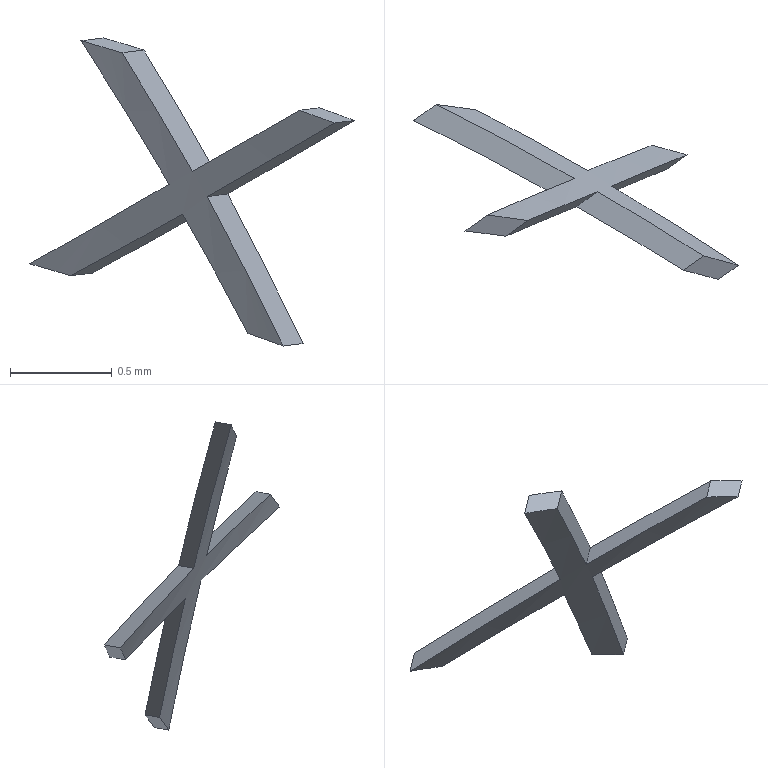Part | SolidWorks | features BaseBody 1 | 1 solid | 14 faces | box 1.595 x 0.8611 x 1.514 mm | volume 0.04844 mm3 | plane 12 | cylinder 2 | commonest cylinder face diameters 16.8 x1 17 x1
STEP:
#1=CARTESIAN_POINT('',(1968.242,-235.583,995.231));
#2=VERTEX_POINT('',#1);
#3=CARTESIAN_POINT('',(1968.793,-235.877,995.534));
#4=VERTEX_POINT('',#3);
#5=CARTESIAN_POINT('',(1968.242,-235.583,995.231));
#6=CARTESIAN_POINT('',(1968.429,-235.677,995.331));
#7=CARTESIAN_POINT('',(1968.612,-235.775,995.432));
#8=CARTESIAN_POINT('',(1968.793,-235.877,995.534));
#9=B_SPLINE_CURVE_WITH_KNOTS('',3,(#5,#6,#7,#8),.UNSPECIFIED.,.F.,.F.,(4,4),(0.,1.),.UNSPECIFIED.);
#10=EDGE_CURVE('',#2,#4,#9,.T.);
#11=ORIENTED_EDGE('',*,*,#10,.T.);
#12=CARTESIAN_POINT('',(1969.113,-235.75,994.948));
#13=VERTEX_POINT('',#12);
#14=CARTESIAN_POINT('',(1968.793,-235.877,995.534));
#15=CARTESIAN_POINT('',(1968.903,-235.832,995.341));
#16=CARTESIAN_POINT('',(1969.01,-235.79,995.145));
#17=CARTESIAN_POINT('',(1969.113,-235.75,994.948));
#18=B_SPLINE_CURVE_WITH_KNOTS('',3,(#14,#15,#16,#17),.UNSPECIFIED.,.F.,.F.,(4,4),(0.,1.),.UNSPECIFIED.);
#19=EDGE_CURVE('',#4,#13,#18,.T.);
#20=ORIENTED_EDGE('',*,*,#19,.T.);
#21=CARTESIAN_POINT('',(1969.287,-235.795,994.885));
#22=VERTEX_POINT('',#21);
#23=CARTESIAN_POINT('',(1966.247,-243.063,991.97));
#24=DIRECTION('',(-0.2015,0.436,-0.8771));
#25=DIRECTION('',(-0.7309,-0.6631,-0.1618));
#26=AXIS2_PLACEMENT_3D('',#23,#24,#25);
#27=CIRCLE('',#26,8.4);
#28=EDGE_CURVE('',#13,#22,#27,.T.);
#29=ORIENTED_EDGE('',*,*,#28,.T.);
#30=CARTESIAN_POINT('',(1968.912,-235.954,995.62));
#31=VERTEX_POINT('',#30);
#32=CARTESIAN_POINT('',(1968.912,-235.954,995.62));
#33=CARTESIAN_POINT('',(1969.042,-235.897,995.379));
#34=CARTESIAN_POINT('',(1969.167,-235.844,995.133));
#35=CARTESIAN_POINT('',(1969.287,-235.795,994.885));
#36=B_SPLINE_CURVE_WITH_KNOTS('',3,(#32,#33,#34,#35),.UNSPECIFIED.,.F.,.F.,(4,4),(0.,1.),.UNSPECIFIED.);
#37=EDGE_CURVE('',#31,#22,#36,.T.);
#38=ORIENTED_EDGE('',*,*,#37,.F.);
#39=CARTESIAN_POINT('',(1969.539,-236.34,995.982));
#40=VERTEX_POINT('',#39);
#41=CARTESIAN_POINT('',(1968.912,-235.954,995.62));
#42=CARTESIAN_POINT('',(1969.125,-236.077,995.74));
#43=CARTESIAN_POINT('',(1969.334,-236.206,995.861));
#44=CARTESIAN_POINT('',(1969.539,-236.34,995.982));
#45=B_SPLINE_CURVE_WITH_KNOTS('',3,(#41,#42,#43,#44),.UNSPECIFIED.,.F.,.F.,(4,4),(0.,1.),.UNSPECIFIED.);
#46=EDGE_CURVE('',#31,#40,#45,.T.);
#47=ORIENTED_EDGE('',*,*,#46,.T.);
#48=CARTESIAN_POINT('',(1969.365,-236.295,996.044));
#49=VERTEX_POINT('',#48);
#50=CARTESIAN_POINT('',(1966.499,-243.608,993.067));
#51=DIRECTION('',(0.2015,-0.436,0.8771));
#52=DIRECTION('',(-0.7309,-0.6631,-0.1618));
#53=AXIS2_PLACEMENT_3D('',#50,#51,#52);
#54=CIRCLE('',#53,8.4);
#55=EDGE_CURVE('',#40,#49,#54,.T.);
#56=ORIENTED_EDGE('',*,*,#55,.T.);
#57=CARTESIAN_POINT('',(1968.841,-235.982,995.744));
#58=VERTEX_POINT('',#57);
#59=CARTESIAN_POINT('',(1968.841,-235.982,995.744));
#60=CARTESIAN_POINT('',(1969.018,-236.082,995.844));
#61=CARTESIAN_POINT('',(1969.193,-236.187,995.944));
#62=CARTESIAN_POINT('',(1969.365,-236.295,996.044));
#63=B_SPLINE_CURVE_WITH_KNOTS('',3,(#59,#60,#61,#62),.UNSPECIFIED.,.F.,.F.,(4,4),(0.,1.),.UNSPECIFIED.);
#64=EDGE_CURVE('',#58,#49,#63,.T.);
#65=ORIENTED_EDGE('',*,*,#64,.F.);
#66=CARTESIAN_POINT('',(1968.494,-236.128,996.327));
#67=VERTEX_POINT('',#66);
#68=CARTESIAN_POINT('',(1968.494,-236.128,996.327));
#69=CARTESIAN_POINT('',(1968.613,-236.076,996.136));
#70=CARTESIAN_POINT('',(1968.729,-236.028,995.941));
#71=CARTESIAN_POINT('',(1968.841,-235.982,995.744));
#72=B_SPLINE_CURVE_WITH_KNOTS('',3,(#68,#69,#70,#71),.UNSPECIFIED.,.F.,.F.,(4,4),(0.,1.),.UNSPECIFIED.);
#73=EDGE_CURVE('',#67,#58,#72,.T.);
#74=ORIENTED_EDGE('',*,*,#73,.F.);
#75=CARTESIAN_POINT('',(1968.293,-236.103,996.386));
#76=VERTEX_POINT('',#75);
#77=CARTESIAN_POINT('',(1966.499,-243.608,993.067));
#78=DIRECTION('',(0.2015,-0.436,0.8771));
#79=DIRECTION('',(-0.7309,-0.6631,-0.1618));
#80=AXIS2_PLACEMENT_3D('',#77,#78,#79);
#81=CIRCLE('',#80,8.4);
#82=EDGE_CURVE('',#67,#76,#81,.T.);
#83=ORIENTED_EDGE('',*,*,#82,.T.);
#84=CARTESIAN_POINT('',(1968.726,-235.918,995.681));
#85=VERTEX_POINT('',#84);
#86=CARTESIAN_POINT('',(1968.293,-236.103,996.386));
#87=CARTESIAN_POINT('',(1968.442,-236.037,996.155));
#88=CARTESIAN_POINT('',(1968.587,-235.975,995.92));
#89=CARTESIAN_POINT('',(1968.726,-235.918,995.681));
#90=B_SPLINE_CURVE_WITH_KNOTS('',3,(#86,#87,#88,#89),.UNSPECIFIED.,.F.,.F.,(4,4),(0.,1.),.UNSPECIFIED.);
#91=EDGE_CURVE('',#76,#85,#90,.T.);
#92=ORIENTED_EDGE('',*,*,#91,.T.);
#93=CARTESIAN_POINT('',(1968.041,-235.558,995.289));
#94=VERTEX_POINT('',#93);
#95=CARTESIAN_POINT('',(1968.041,-235.558,995.289));
#96=CARTESIAN_POINT('',(1968.273,-235.671,995.419));
#97=CARTESIAN_POINT('',(1968.502,-235.791,995.55));
#98=CARTESIAN_POINT('',(1968.726,-235.918,995.681));
#99=B_SPLINE_CURVE_WITH_KNOTS('',3,(#95,#96,#97,#98),.UNSPECIFIED.,.F.,.F.,(4,4),(0.,1.),.UNSPECIFIED.);
#100=EDGE_CURVE('',#94,#85,#99,.T.);
#101=ORIENTED_EDGE('',*,*,#100,.F.);
#102=CARTESIAN_POINT('',(1966.247,-243.063,991.97));
#103=DIRECTION('',(-0.2015,0.436,-0.8771));
#104=DIRECTION('',(-0.7309,-0.6631,-0.1618));
#105=AXIS2_PLACEMENT_3D('',#102,#103,#104);
#106=CIRCLE('',#105,8.4);
#107=EDGE_CURVE('',#94,#2,#106,.T.);
#108=ORIENTED_EDGE('',*,*,#107,.T.);
#109=EDGE_LOOP('',(#11,#20,#29,#38,#47,#56,#65,#74,#83,#92,#101,#108));
#110=FACE_OUTER_BOUND('',#109,.T.);
#111=CARTESIAN_POINT('',(1967.45,-245.666,997.207));
#112=DIRECTION('',(0.2015,-0.436,0.8771));
#113=DIRECTION('',(-0.7309,-0.6631,-0.1618));
#114=AXIS2_PLACEMENT_3D('',#111,#112,#113);
#115=CYLINDRICAL_SURFACE('',#114,8.4);
#116=ADVANCED_FACE('',(#110),#115,.F.);
#117=CARTESIAN_POINT('',(1968.35,-235.506,995.244));
#118=VERTEX_POINT('',#117);
#119=CARTESIAN_POINT('',(1968.296,-235.544,995.237));
#120=DIRECTION('',(-0.8088,-0.5792,-0.1022));
#121=VECTOR('',#120,1000.);
#122=LINE('',#119,#121);
#123=EDGE_CURVE('',#118,#2,#122,.T.);
#124=ORIENTED_EDGE('',*,*,#123,.T.);
#125=ORIENTED_EDGE('',*,*,#107,.F.);
#126=CARTESIAN_POINT('',(1968.151,-235.479,995.303));
#127=VERTEX_POINT('',#126);
#128=CARTESIAN_POINT('',(1968.096,-235.518,995.296));
#129=DIRECTION('',(-0.8088,-0.5792,-0.1022));
#130=VECTOR('',#129,1000.);
#131=LINE('',#128,#130);
#132=EDGE_CURVE('',#127,#94,#131,.T.);
#133=ORIENTED_EDGE('',*,*,#132,.F.);
#134=CARTESIAN_POINT('',(1966.247,-243.063,991.97));
#135=DIRECTION('',(-0.2015,0.436,-0.8771));
#136=DIRECTION('',(-0.7309,-0.6631,-0.1618));
#137=AXIS2_PLACEMENT_3D('',#134,#135,#136);
#138=CIRCLE('',#137,8.5);
#139=EDGE_CURVE('',#127,#118,#138,.T.);
#140=ORIENTED_EDGE('',*,*,#139,.T.);
#141=EDGE_LOOP('',(#124,#125,#133,#140));
#142=FACE_OUTER_BOUND('',#141,.T.);
#143=CARTESIAN_POINT('',(1981.656,-238.46,990.719));
#144=DIRECTION('',(-0.2015,0.436,-0.8771));
#145=DIRECTION('',(-0.5526,0.6888,0.4693));
#146=AXIS2_PLACEMENT_3D('',#143,#144,#145);
#147=PLANE('',#146);
#148=ADVANCED_FACE('',(#142),#147,.T.);
#149=ORIENTED_EDGE('',*,*,#132,.T.);
#150=ORIENTED_EDGE('',*,*,#100,.T.);
#151=CARTESIAN_POINT('',(1968.83,-235.843,995.694));
#152=VERTEX_POINT('',#151);
#153=CARTESIAN_POINT('',(1968.778,-235.881,995.687));
#154=DIRECTION('',(-0.8088,-0.5792,-0.1022));
#155=VECTOR('',#154,1000.);
#156=LINE('',#153,#155);
#157=EDGE_CURVE('',#152,#85,#156,.T.);
#158=ORIENTED_EDGE('',*,*,#157,.F.);
#159=CARTESIAN_POINT('',(1968.151,-235.479,995.303));
#160=CARTESIAN_POINT('',(1968.289,-235.548,995.381));
#161=CARTESIAN_POINT('',(1968.426,-235.619,995.459));
#162=CARTESIAN_POINT('',(1968.562,-235.692,995.537));
#163=CARTESIAN_POINT('',(1968.696,-235.767,995.615));
#164=CARTESIAN_POINT('',(1968.83,-235.843,995.694));
#165=B_SPLINE_CURVE_WITH_KNOTS('',5,(#159,#160,#161,#162,#163,#164),.UNSPECIFIED.,.F.,.F.,(6,6),(0.,1.),.UNSPECIFIED.);
#166=EDGE_CURVE('',#127,#152,#165,.T.);
#167=ORIENTED_EDGE('',*,*,#166,.F.);
#168=EDGE_LOOP('',(#149,#150,#158,#167));
#169=FACE_OUTER_BOUND('',#168,.T.);
#170=CARTESIAN_POINT('',(1975.582,-231.008,996.547));
#171=DIRECTION('',(-0.3392,0.3175,0.8855));
#172=DIRECTION('',(0.4805,-0.7508,0.4532));
#173=AXIS2_PLACEMENT_3D('',#170,#171,#172);
#174=PLANE('',#173);
#175=ADVANCED_FACE('',(#169),#174,.T.);
#176=ORIENTED_EDGE('',*,*,#157,.T.);
#177=ORIENTED_EDGE('',*,*,#91,.F.);
#178=CARTESIAN_POINT('',(1968.403,-236.024,996.4));
#179=VERTEX_POINT('',#178);
#180=CARTESIAN_POINT('',(1968.348,-236.064,996.393));
#181=DIRECTION('',(-0.8088,-0.5792,-0.1022));
#182=VECTOR('',#181,1000.);
#183=LINE('',#180,#182);
#184=EDGE_CURVE('',#179,#76,#183,.T.);
#185=ORIENTED_EDGE('',*,*,#184,.F.);
#186=CARTESIAN_POINT('',(1968.403,-236.024,996.4));
#187=CARTESIAN_POINT('',(1968.491,-235.985,996.261));
#188=CARTESIAN_POINT('',(1968.578,-235.948,996.121));
#189=CARTESIAN_POINT('',(1968.664,-235.912,995.98));
#190=CARTESIAN_POINT('',(1968.747,-235.877,995.838));
#191=CARTESIAN_POINT('',(1968.83,-235.843,995.694));
#192=B_SPLINE_CURVE_WITH_KNOTS('',5,(#186,#187,#188,#189,#190,#191),.UNSPECIFIED.,.F.,.F.,(6,6),(0.,1.),.UNSPECIFIED.);
#193=EDGE_CURVE('',#179,#152,#192,.T.);
#194=ORIENTED_EDGE('',*,*,#193,.T.);
#195=EDGE_LOOP('',(#176,#177,#185,#194));
#196=FACE_OUTER_BOUND('',#195,.T.);
#197=CARTESIAN_POINT('',(1975.461,-230.969,997.291));
#198=DIRECTION('',(-0.5657,0.8136,-0.134));
#199=DIRECTION('',(-0.1608,0.05058,0.9857));
#200=AXIS2_PLACEMENT_3D('',#197,#198,#199);
#201=PLANE('',#200);
#202=ADVANCED_FACE('',(#196),#201,.T.);
#203=ORIENTED_EDGE('',*,*,#184,.T.);
#204=ORIENTED_EDGE('',*,*,#82,.F.);
#205=CARTESIAN_POINT('',(1968.602,-236.051,996.341));
#206=VERTEX_POINT('',#205);
#207=CARTESIAN_POINT('',(1968.548,-236.09,996.334));
#208=DIRECTION('',(-0.8088,-0.5792,-0.1022));
#209=VECTOR('',#208,1000.);
#210=LINE('',#207,#209);
#211=EDGE_CURVE('',#206,#67,#210,.T.);
#212=ORIENTED_EDGE('',*,*,#211,.F.);
#213=CARTESIAN_POINT('',(1966.499,-243.608,993.067));
#214=DIRECTION('',(0.2015,-0.436,0.8771));
#215=DIRECTION('',(-0.7309,-0.6631,-0.1618));
#216=AXIS2_PLACEMENT_3D('',#213,#214,#215);
#217=CIRCLE('',#216,8.5);
#218=EDGE_CURVE('',#206,#179,#217,.T.);
#219=ORIENTED_EDGE('',*,*,#218,.T.);
#220=EDGE_LOOP('',(#203,#204,#212,#219));
#221=FACE_OUTER_BOUND('',#220,.T.);
#222=CARTESIAN_POINT('',(1982.253,-239.435,991.522));
#223=DIRECTION('',(0.2015,-0.436,0.8771));
#224=DIRECTION('',(0.5526,-0.6888,-0.4693));
#225=AXIS2_PLACEMENT_3D('',#222,#223,#224);
#226=PLANE('',#225);
#227=ADVANCED_FACE('',(#221),#226,.T.);
#228=ORIENTED_EDGE('',*,*,#211,.T.);
#229=ORIENTED_EDGE('',*,*,#73,.T.);
#230=CARTESIAN_POINT('',(1968.944,-235.908,995.757));
#231=VERTEX_POINT('',#230);
#232=CARTESIAN_POINT('',(1968.893,-235.945,995.75));
#233=DIRECTION('',(-0.8088,-0.5792,-0.1022));
#234=VECTOR('',#233,1000.);
#235=LINE('',#232,#234);
#236=EDGE_CURVE('',#231,#58,#235,.T.);
#237=ORIENTED_EDGE('',*,*,#236,.F.);
#238=CARTESIAN_POINT('',(1968.602,-236.051,996.341));
#239=CARTESIAN_POINT('',(1968.672,-236.021,996.226));
#240=CARTESIAN_POINT('',(1968.742,-235.991,996.11));
#241=CARTESIAN_POINT('',(1968.81,-235.963,995.993));
#242=CARTESIAN_POINT('',(1968.878,-235.935,995.875));
#243=CARTESIAN_POINT('',(1968.944,-235.908,995.757));
#244=B_SPLINE_CURVE_WITH_KNOTS('',5,(#238,#239,#240,#241,#242,#243),.UNSPECIFIED.,.F.,.F.,(6,6),(0.,1.),.UNSPECIFIED.);
#245=EDGE_CURVE('',#206,#231,#244,.T.);
#246=ORIENTED_EDGE('',*,*,#245,.F.);
#247=EDGE_LOOP('',(#228,#229,#237,#246));
#248=FACE_OUTER_BOUND('',#247,.T.);
#249=CARTESIAN_POINT('',(1975.647,-231.108,996.604));
#250=DIRECTION('',(0.566,-0.8137,0.1326));
#251=DIRECTION('',(0.1599,-0.04938,-0.9859));
#252=AXIS2_PLACEMENT_3D('',#249,#250,#251);
#253=PLANE('',#252);
#254=ADVANCED_FACE('',(#248),#253,.T.);
#255=ORIENTED_EDGE('',*,*,#236,.T.);
#256=ORIENTED_EDGE('',*,*,#64,.T.);
#257=CARTESIAN_POINT('',(1969.464,-236.224,996.056));
#258=VERTEX_POINT('',#257);
#259=CARTESIAN_POINT('',(1969.415,-236.26,996.05));
#260=DIRECTION('',(-0.8088,-0.5792,-0.1022));
#261=VECTOR('',#260,1000.);
#262=LINE('',#259,#261);
#263=EDGE_CURVE('',#258,#49,#262,.T.);
#264=ORIENTED_EDGE('',*,*,#263,.F.);
#265=CARTESIAN_POINT('',(1968.944,-235.908,995.757));
#266=CARTESIAN_POINT('',(1969.05,-235.969,995.817));
#267=CARTESIAN_POINT('',(1969.154,-236.031,995.876));
#268=CARTESIAN_POINT('',(1969.258,-236.094,995.936));
#269=CARTESIAN_POINT('',(1969.362,-236.159,995.996));
#270=CARTESIAN_POINT('',(1969.464,-236.224,996.056));
#271=B_SPLINE_CURVE_WITH_KNOTS('',5,(#265,#266,#267,#268,#269,#270),.UNSPECIFIED.,.F.,.F.,(6,6),(0.,1.),.UNSPECIFIED.);
#272=EDGE_CURVE('',#231,#258,#271,.T.);
#273=ORIENTED_EDGE('',*,*,#272,.F.);
#274=EDGE_LOOP('',(#255,#256,#264,#273));
#275=FACE_OUTER_BOUND('',#274,.T.);
#276=CARTESIAN_POINT('',(1975.95,-231.579,996.876));
#277=DIRECTION('',(-0.3302,0.3034,0.8938));
#278=DIRECTION('',(0.4867,-0.7566,0.4367));
#279=AXIS2_PLACEMENT_3D('',#276,#277,#278);
#280=PLANE('',#279);
#281=ADVANCED_FACE('',(#275),#280,.T.);
#282=ORIENTED_EDGE('',*,*,#263,.T.);
#283=ORIENTED_EDGE('',*,*,#55,.F.);
#284=CARTESIAN_POINT('',(1969.636,-236.27,995.994));
#285=VERTEX_POINT('',#284);
#286=CARTESIAN_POINT('',(1969.587,-236.305,995.988));
#287=DIRECTION('',(-0.8088,-0.5792,-0.1022));
#288=VECTOR('',#287,1000.);
#289=LINE('',#286,#288);
#290=EDGE_CURVE('',#285,#40,#289,.T.);
#291=ORIENTED_EDGE('',*,*,#290,.F.);
#292=CARTESIAN_POINT('',(1966.499,-243.608,993.067));
#293=DIRECTION('',(0.2015,-0.436,0.8771));
#294=DIRECTION('',(-0.7309,-0.6631,-0.1618));
#295=AXIS2_PLACEMENT_3D('',#292,#293,#294);
#296=CIRCLE('',#295,8.5);
#297=EDGE_CURVE('',#285,#258,#296,.T.);
#298=ORIENTED_EDGE('',*,*,#297,.T.);
#299=EDGE_LOOP('',(#282,#283,#291,#298));
#300=FACE_OUTER_BOUND('',#299,.T.);
#301=CARTESIAN_POINT('',(1982.253,-239.435,991.522));
#302=DIRECTION('',(0.2015,-0.436,0.8771));
#303=DIRECTION('',(0.5526,-0.6888,-0.4693));
#304=AXIS2_PLACEMENT_3D('',#301,#302,#303);
#305=PLANE('',#304);
#306=ADVANCED_FACE('',(#300),#305,.T.);
#307=ORIENTED_EDGE('',*,*,#290,.T.);
#308=ORIENTED_EDGE('',*,*,#46,.F.);
#309=CARTESIAN_POINT('',(1969.014,-235.881,995.633));
#310=VERTEX_POINT('',#309);
#311=CARTESIAN_POINT('',(1968.963,-235.917,995.627));
#312=DIRECTION('',(-0.8088,-0.5792,-0.1022));
#313=VECTOR('',#312,1000.);
#314=LINE('',#311,#313);
#315=EDGE_CURVE('',#310,#31,#314,.T.);
#316=ORIENTED_EDGE('',*,*,#315,.F.);
#317=CARTESIAN_POINT('',(1969.014,-235.881,995.633));
#318=CARTESIAN_POINT('',(1969.141,-235.955,995.705));
#319=CARTESIAN_POINT('',(1969.266,-236.032,995.777));
#320=CARTESIAN_POINT('',(1969.391,-236.11,995.849));
#321=CARTESIAN_POINT('',(1969.514,-236.189,995.922));
#322=CARTESIAN_POINT('',(1969.636,-236.27,995.994));
#323=B_SPLINE_CURVE_WITH_KNOTS('',5,(#317,#318,#319,#320,#321,#322),.UNSPECIFIED.,.F.,.F.,(6,6),(0.,1.),.UNSPECIFIED.);
#324=EDGE_CURVE('',#310,#285,#323,.T.);
#325=ORIENTED_EDGE('',*,*,#324,.T.);
#326=EDGE_LOOP('',(#307,#308,#316,#325));
#327=FACE_OUTER_BOUND('',#326,.T.);
#328=CARTESIAN_POINT('',(1975.669,-231.115,996.474));
#329=DIRECTION('',(0.3295,-0.3023,-0.8944));
#330=DIRECTION('',(-0.4872,0.7571,-0.4354));
#331=AXIS2_PLACEMENT_3D('',#328,#329,#330);
#332=PLANE('',#331);
#333=ADVANCED_FACE('',(#327),#332,.T.);
#334=ORIENTED_EDGE('',*,*,#315,.T.);
#335=ORIENTED_EDGE('',*,*,#37,.T.);
#336=CARTESIAN_POINT('',(1969.384,-235.725,994.898));
#337=VERTEX_POINT('',#336);
#338=CARTESIAN_POINT('',(1969.336,-235.76,994.891));
#339=DIRECTION('',(-0.8088,-0.5792,-0.1022));
#340=VECTOR('',#339,1000.);
#341=LINE('',#338,#340);
#342=EDGE_CURVE('',#337,#22,#341,.T.);
#343=ORIENTED_EDGE('',*,*,#342,.F.);
#344=CARTESIAN_POINT('',(1969.014,-235.881,995.633));
#345=CARTESIAN_POINT('',(1969.091,-235.848,995.488));
#346=CARTESIAN_POINT('',(1969.166,-235.815,995.342));
#347=CARTESIAN_POINT('',(1969.24,-235.784,995.194));
#348=CARTESIAN_POINT('',(1969.313,-235.754,995.046));
#349=CARTESIAN_POINT('',(1969.384,-235.725,994.898));
#350=B_SPLINE_CURVE_WITH_KNOTS('',5,(#344,#345,#346,#347,#348,#349),.UNSPECIFIED.,.F.,.F.,(6,6),(0.,1.),.UNSPECIFIED.);
#351=EDGE_CURVE('',#310,#337,#350,.T.);
#352=ORIENTED_EDGE('',*,*,#351,.F.);
#353=EDGE_LOOP('',(#334,#335,#343,#352));
#354=FACE_OUTER_BOUND('',#353,.T.);
#355=CARTESIAN_POINT('',(1975.785,-231.142,995.706));
#356=DIRECTION('',(0.5689,-0.8145,0.1142));
#357=DIRECTION('',(0.1494,-0.03424,-0.9882));
#358=AXIS2_PLACEMENT_3D('',#355,#356,#357);
#359=PLANE('',#358);
#360=ADVANCED_FACE('',(#354),#359,.T.);
#361=ORIENTED_EDGE('',*,*,#342,.T.);
#362=ORIENTED_EDGE('',*,*,#28,.F.);
#363=CARTESIAN_POINT('',(1969.212,-235.679,994.96));
#364=VERTEX_POINT('',#363);
#365=CARTESIAN_POINT('',(1969.163,-235.715,994.954));
#366=DIRECTION('',(-0.8088,-0.5792,-0.1022));
#367=VECTOR('',#366,1000.);
#368=LINE('',#365,#367);
#369=EDGE_CURVE('',#364,#13,#368,.T.);
#370=ORIENTED_EDGE('',*,*,#369,.F.);
#371=CARTESIAN_POINT('',(1966.247,-243.063,991.97));
#372=DIRECTION('',(-0.2015,0.436,-0.8771));
#373=DIRECTION('',(-0.7309,-0.6631,-0.1618));
#374=AXIS2_PLACEMENT_3D('',#371,#372,#373);
#375=CIRCLE('',#374,8.5);
#376=EDGE_CURVE('',#364,#337,#375,.T.);
#377=ORIENTED_EDGE('',*,*,#376,.T.);
#378=EDGE_LOOP('',(#361,#362,#370,#377));
#379=FACE_OUTER_BOUND('',#378,.T.);
#380=CARTESIAN_POINT('',(1981.656,-238.46,990.719));
#381=DIRECTION('',(-0.2015,0.436,-0.8771));
#382=DIRECTION('',(-0.5526,0.6888,0.4693));
#383=AXIS2_PLACEMENT_3D('',#380,#381,#382);
#384=PLANE('',#383);
#385=ADVANCED_FACE('',(#379),#384,.T.);
#386=ORIENTED_EDGE('',*,*,#369,.T.);
#387=ORIENTED_EDGE('',*,*,#19,.F.);
#388=CARTESIAN_POINT('',(1968.896,-235.804,995.547));
#389=VERTEX_POINT('',#388);
#390=CARTESIAN_POINT('',(1968.844,-235.841,995.541));
#391=DIRECTION('',(-0.8088,-0.5792,-0.1022));
#392=VECTOR('',#391,1000.);
#393=LINE('',#390,#392);
#394=EDGE_CURVE('',#389,#4,#393,.T.);
#395=ORIENTED_EDGE('',*,*,#394,.F.);
#396=CARTESIAN_POINT('',(1968.896,-235.804,995.547));
#397=CARTESIAN_POINT('',(1968.961,-235.777,995.431));
#398=CARTESIAN_POINT('',(1969.025,-235.752,995.314));
#399=CARTESIAN_POINT('',(1969.088,-235.727,995.197));
#400=CARTESIAN_POINT('',(1969.151,-235.703,995.079));
#401=CARTESIAN_POINT('',(1969.212,-235.679,994.96));
#402=B_SPLINE_CURVE_WITH_KNOTS('',5,(#396,#397,#398,#399,#400,#401),.UNSPECIFIED.,.F.,.F.,(6,6),(0.,1.),.UNSPECIFIED.);
#403=EDGE_CURVE('',#389,#364,#402,.T.);
#404=ORIENTED_EDGE('',*,*,#403,.T.);
#405=EDGE_LOOP('',(#386,#387,#395,#404));
#406=FACE_OUTER_BOUND('',#405,.T.);
#407=CARTESIAN_POINT('',(1975.599,-231.003,996.394));
#408=DIRECTION('',(-0.566,0.8137,-0.1326));
#409=DIRECTION('',(-0.1599,0.04938,0.9859));
#410=AXIS2_PLACEMENT_3D('',#407,#408,#409);
#411=PLANE('',#410);
#412=ADVANCED_FACE('',(#406),#411,.T.);
#413=ORIENTED_EDGE('',*,*,#394,.T.);
#414=ORIENTED_EDGE('',*,*,#10,.F.);
#415=ORIENTED_EDGE('',*,*,#123,.F.);
#416=CARTESIAN_POINT('',(1968.35,-235.506,995.244));
#417=CARTESIAN_POINT('',(1968.461,-235.563,995.305));
#418=CARTESIAN_POINT('',(1968.571,-235.621,995.365));
#419=CARTESIAN_POINT('',(1968.68,-235.681,995.425));
#420=CARTESIAN_POINT('',(1968.788,-235.742,995.486));
#421=CARTESIAN_POINT('',(1968.896,-235.804,995.547));
#422=B_SPLINE_CURVE_WITH_KNOTS('',5,(#416,#417,#418,#419,#420,#421),.UNSPECIFIED.,.F.,.F.,(6,6),(0.,1.),.UNSPECIFIED.);
#423=EDGE_CURVE('',#118,#389,#422,.T.);
#424=ORIENTED_EDGE('',*,*,#423,.T.);
#425=EDGE_LOOP('',(#413,#414,#415,#424));
#426=FACE_OUTER_BOUND('',#425,.T.);
#427=CARTESIAN_POINT('',(1975.295,-230.532,996.122));
#428=DIRECTION('',(0.3302,-0.3034,-0.8938));
#429=DIRECTION('',(-0.4867,0.7566,-0.4367));
#430=AXIS2_PLACEMENT_3D('',#427,#428,#429);
#431=PLANE('',#430);
#432=ADVANCED_FACE('',(#426),#431,.T.);
#433=ORIENTED_EDGE('',*,*,#139,.F.);
#434=ORIENTED_EDGE('',*,*,#166,.T.);
#435=ORIENTED_EDGE('',*,*,#193,.F.);
#436=ORIENTED_EDGE('',*,*,#218,.F.);
#437=ORIENTED_EDGE('',*,*,#245,.T.);
#438=ORIENTED_EDGE('',*,*,#272,.T.);
#439=ORIENTED_EDGE('',*,*,#297,.F.);
#440=ORIENTED_EDGE('',*,*,#324,.F.);
#441=ORIENTED_EDGE('',*,*,#351,.T.);
#442=ORIENTED_EDGE('',*,*,#376,.F.);
#443=ORIENTED_EDGE('',*,*,#403,.F.);
#444=ORIENTED_EDGE('',*,*,#423,.F.);
#445=EDGE_LOOP('',(#433,#434,#435,#436,#437,#438,#439,#440,#441,#442,#443,#444));
#446=FACE_OUTER_BOUND('',#445,.T.);
#447=CARTESIAN_POINT('',(1967.45,-245.666,997.207));
#448=DIRECTION('',(0.2015,-0.436,0.8771));
#449=DIRECTION('',(-0.7309,-0.6631,-0.1618));
#450=AXIS2_PLACEMENT_3D('',#447,#448,#449);
#451=CYLINDRICAL_SURFACE('',#450,8.5);
#452=ADVANCED_FACE('',(#446),#451,.T.);
#453=CLOSED_SHELL('',(#116,#148,#175,#202,#227,#254,#281,#306,#333,#360,#385,#412,#432,#452));
#454=MANIFOLD_SOLID_BREP('',#453);
#455=CARTESIAN_POINT('',(0.,0.,0.));
#456=DIRECTION('',(0.,0.,1.));
#457=DIRECTION('',(1.,0.,0.));
#458=AXIS2_PLACEMENT_3D('',#455,#456,#457);
#459=(LENGTH_UNIT()NAMED_UNIT(*)SI_UNIT(.MILLI.,.METRE.));
#460=UNCERTAINTY_MEASURE_WITH_UNIT(LENGTH_MEASURE(0.00001),#459,'','');
#461=(NAMED_UNIT(*)PLANE_ANGLE_UNIT()SI_UNIT($,.RADIAN.));
#462=(NAMED_UNIT(*)SI_UNIT($,.STERADIAN.)SOLID_ANGLE_UNIT());
#463=(GEOMETRIC_REPRESENTATION_CONTEXT(3)GLOBAL_UNCERTAINTY_ASSIGNED_CONTEXT((#460))GLOBAL_UNIT_ASSIGNED_CONTEXT((#459,#461,#462))REPRESENTATION_CONTEXT('',''));
#464=ADVANCED_BREP_SHAPE_REPRESENTATION('',(#454,#458),#463);